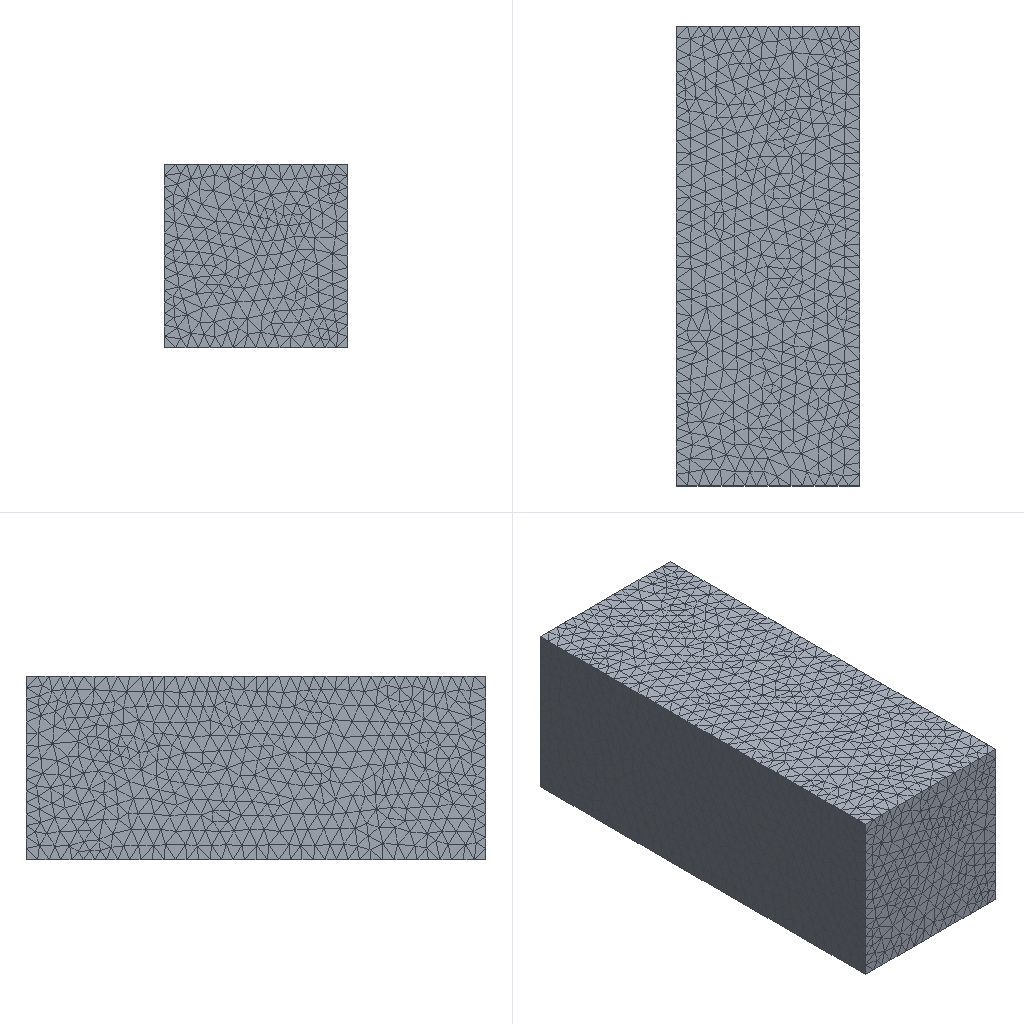Simulation study | ansys workbench
Set-up summary:
category,name,step,type,value,unit,region
solver,ansys_workbench
units,mm-N-s-tonne (MPa),,stated,"/units,MPA"
analysis,LS1,,static
load_step,LS1,LS1,static,nsubst=1; time=1
mesh,nodes,,,44583
mesh,elements,,,30476
element_type,SOLID187,,,22294
element_type,TARGE170,,,3416
element_type,CONTA174,,,3416
element_type,SOLID186,,,948
element_type,SURF154,,,402
material,"? , ABS ( ? )",,E,1628,tonne s^-2 mm^-1
material,"? , ABS ( ? )",,nu,0.4089
material,"? , ABS ( ? )",,density,1.03e-09,tonne mm^-3
material,"? , ABS ( ? )",,conductivity,0.1997,tonne mm s^-3 C^-1
material,"? , ABS ( ? )",,specific_heat,1.4e+09,mm^2 s^-2 C^-1
material,"? , ABS ( ? )",,cte,0.000184,C^-1
material,"? , EN GJL 100",,E,89440,tonne s^-2 mm^-1
material,"? , EN GJL 100",,nu,0.26
material,"? , EN GJL 100",,density,6.999e-09,tonne mm^-3
material,"? , EN GJL 100",,conductivity,60,tonne mm s^-3 C^-1
material,"? , EN GJL 100",,specific_heat,4.996e+08,mm^2 s^-2 C^-1
material,"? , EN GJL 100",,cte,1.196e-05,C^-1
load,Define Force Using Surface Effect Elements,LS1,surface-effect pres face 2,-0.0003125,,SURF154 #15
bc,Fixed Supports,model,fixed,[dofs=ALL],,_FIXEDSU
bc,"Elements for Body 1 ""________|NONE""",model,fixed,[dofs=ALL n=3],,node list
bc,"Elements for Body 2 ""____|____-____1""",model,fixed,[dofs=ALL n=3],,node list
contact,Frictional - ____|____-____1 ? ________|NONE,,standard (frictionless/frictional),friction=0.2; element=CONTA174
contact,Frictional - ____|____-____1 ? ________|NONE,,standard (frictionless/frictional),friction=0.2; element=CONTA174
contact,Frictional - ____|____-____1 ? ________|NONE,,standard (frictionless/frictional),friction=0.2; element=CONTA174
contact,Frictional - ____|____-____1 ? ________|NONE,,standard (frictionless/frictional),friction=0.2; element=CONTA174
contact,Frictional - ____|____-____1 ? ________|NONE,,standard (frictionless/frictional),friction=0.2; element=CONTA174
contact,Frictional - ____|____-____1 ? ________|NONE,,standard (frictionless/frictional),friction=0.2; element=CONTA174
named_set,_FIXEDSU,,node,877
Ansys APDL input file, long lists of numbers shortened:
/batch
/config,noeldb,1     ! force off writing results to database
*get,_wallstrt,active,,time,wall
! ANSYS input file written by Workbench version 2021 R1
! File used for geometry attach:
/title,wbnew--____ (A5)
! ****** Begin Custom Load Command Snippet ******
/COM, ACT Extensions:
/COM,     LSDYNA, 2021.1
/COM,
! ****** End   Custom Load Command Snippet ******
*DIM,_wb_ProjectScratch_dir,string,248
_wb_ProjectScratch_dir(1) = ''
*DIM,_wb_SolverFiles_dir,string,248
_wb_SolverFiles_dir(1) = ''
*DIM,_wb_userfiles_dir,string,248
_wb_userfiles_dir(1) = ''
/com,--- Data in consistent NMM units. See Solving Units in the help system for more information.
/units,MPA
/nopr
/wb,file,start              !  signify a WB generated input file
/prep7
! Turn off shape checking because checks already performed inside WB mesher.
! See help system for more information.
SHPP,OFF,,NOWARN
/nolist
etcon,set             ! allow ANSYS to choose best KEYOP's for 180x elements, resets any applicable keyopt to MAPDL defaults
/com,*********** Nodes for the whole assembly ***********
nblock,3,,49041
(1i9,3e20.9e3)
        1     2.921746114E+01     1.392875542E+01     3.000000000E+01
! (44582 more lines like these left out)
-1
/wb,elem,start            !  set before creation of elements
/com,*********** Elements for Body 1 "________|NONE" ***********
et,1,187
eblock,19,solid,,22294
(19i9)
        1        1        1        1        0        0        0        0       10        0      949     8227     8267    12768    12354    21057    21282    21066    21062
! (44587 more lines like these left out)
-1
/com,*********** Elements for Body 2 "____|____-____1" ***********
et,2,186
keyo,2,2,1          ! set full integration on SOLID186
eblock,19,solid,,948
(19i9)
        2        2        2        2        0        0        0        0       20        0        1     1022     1133     1122     1110     1108     1144     1121     1109
! (1895 more lines like these left out)
-1
/wb,elem,end               !  done creating elements
/com,*********** Send User Defined Coordinate System(s) ***********
csys,0
toffst,273.15,  ! Temperature offset from absolute zero
/com,*********** Set Reference Temperature ***********
tref,22.
/wb,mat,start              !  starting to send materials
/com,*********** Send Materials ***********
Temperature = 'TEMP' ! Temperature
MP,DENS,1,1.03e-09,	! tonne mm^-3
MP,EX,1,1628,	! tonne s^-2 mm^-1
MP,NUXY,1,0.4089,
MP,ALPX,1,0.000184,	! C^-1
MP,KXX,1,0.1997,	! tonne mm s^-3 C^-1
MP,C,1,1400000000,	! mm^2 s^-2 C^-1
Temperature = 'TEMP' ! Temperature
MP,DENS,2,6.999e-09,	! tonne mm^-3
MP,EX,2,89440,	! tonne s^-2 mm^-1
MP,NUXY,2,0.26,
MP,ALPX,2,1.196e-05,	! C^-1
MP,KXX,2,60,	! tonne mm s^-3 C^-1
MP,C,2,499600000,	! mm^2 s^-2 C^-1
/wb,mat,end                !  done sending materials
!************************* Model Summary ********************
!________|NONE,	塑性，ABS（高冲击）,	matid,	1
!____|____-____1,	铸铁，EN GJL 100,	matid,	2
!************************* End Model Summary ********************
! get the diagonal of the bounding box. Needed later for other things
*get,_xmin,node,,mnloc,x
*get,_ymin,node,,mnloc,y
*get,_zmin,node,,mnloc,z
*get,_xmax,node,,mxloc,x
*get,_ymax,node,,mxloc,y
*get,_zmax,node,,mxloc,z
_ASMDIAG=(_xmax-_xmin)*(_xmax-_xmin)+(_ymax-_ymin)*(_ymax-_ymin)+(_zmax-_zmin)*(_zmax-_zmin)
_ASMDIAG=SQRT(_ASMDIAG)
/wb,contact,start          !  starting to send contact
/com,*********** Create Contact "摩擦的 - ____|____-____1 至 ________|NONE" ***********
/com,            Real Constant Set For Above Contact Is 4 & 3
*set,tid,4
*set,cid,3
r,tid
r,cid
et,tid,170
et,cid,174
eblock,10,,,12
(15i9)
    33019        4        4        4        0     2080      184      160       77     2548     2478     2310     2311
! (11 more lines like these left out)
-1
eblock,10,,,12
(15i9)
    33031        3        3        3        0     2080      184      160       77     2548     2478     2310     2311
! (11 more lines like these left out)
-1
eblock,10,,,226
(15i9)
    33043        3        4        3        0     8203     8226     8229     8229    20864    21048     8229    20865
! (225 more lines like these left out)
-1
eblock,10,,,226
(15i9)
    33269        4        3        4        0     8203     8226     8229     8229    20864    21048     8229    20865
! (225 more lines like these left out)
-1
keyo,cid,8,2               ! auto create asymmetric contact (from Program Controlled setting)
keyo,cid,10,0              ! adjust contact stiffness each NR iteration (from Program Controlled setting)
keyo,cid,12,0              ! standard contact
mp,mu,cid,0.2       ! unitless
keyo,cid,18,1              ! small sliding turned on by application
keyo,cid,2,0               ! augmented Lagrange (from Program Controlled setting)
keyo,cid,4,0               ! on Gauss point (from Program Controlled setting)
keyo,cid,9,0               ! use real geometry with stepped effects
keyo,cid,7,0               ! No Prediction
rmod,tid,3,1.       ! FKN
rmod,tid,5,0.       ! ICONT
rmod,tid,6,0.       ! PINB
rmod,tid,10,0.      ! CNOF
rmod,tid,12,0.      ! FKT
rmod,tid,36,35      ! WB DSID
rmod,cid,3,1.       ! FKN
rmod,cid,5,0.       ! ICONT
rmod,cid,6,0.       ! PINB
rmod,cid,10,0.      ! CNOF
rmod,cid,12,0.      ! FKT
rmod,cid,36,35      ! WB DSID
/com,*********** Create Contact "摩擦的 - ____|____-____1 至 ________|NONE" ***********
/com,            Real Constant Set For Above Contact Is 6 & 5
*set,tid,6
*set,cid,5
r,tid
r,cid
et,tid,170
et,cid,174
eblock,10,,,24
(15i9)
    33495        6        6        6        0      159      161      196      158     2477     2481     2475     2474
! (23 more lines like these left out)
-1
eblock,10,,,24
(15i9)
    33519        5        5        5        0      159      161      196      158     2477     2481     2475     2474
! (23 more lines like these left out)
-1
eblock,10,,,688
(15i9)
    33543        5        6        5        0     8298     8346     8508     8508    21484    21933     8508    21488
! (687 more lines like these left out)
-1
eblock,10,,,688
(15i9)
    34231        6        5        6        0     8298     8346     8508     8508    21484    21933     8508    21488
! (687 more lines like these left out)
-1
keyo,cid,8,2               ! auto create asymmetric contact (from Program Controlled setting)
keyo,cid,10,0              ! adjust contact stiffness each NR iteration (from Program Controlled setting)
keyo,cid,12,0              ! standard contact
mp,mu,cid,0.2       ! unitless
keyo,cid,18,1              ! small sliding turned on by application
keyo,cid,2,0               ! augmented Lagrange (from Program Controlled setting)
keyo,cid,4,0               ! on Gauss point (from Program Controlled setting)
keyo,cid,9,0               ! use real geometry with stepped effects
keyo,cid,7,0               ! No Prediction
rmod,tid,3,1.       ! FKN
rmod,tid,5,0.       ! ICONT
rmod,tid,6,0.       ! PINB
rmod,tid,10,0.      ! CNOF
rmod,tid,12,0.      ! FKT
rmod,tid,36,38      ! WB DSID
rmod,cid,3,1.       ! FKN
rmod,cid,5,0.       ! ICONT
rmod,cid,6,0.       ! PINB
rmod,cid,10,0.      ! CNOF
rmod,cid,12,0.      ! FKT
rmod,cid,36,38      ! WB DSID
/com,*********** Create Contact "摩擦的 - ____|____-____1 至 ________|NONE" ***********
/com,            Real Constant Set For Above Contact Is 8 & 7
*set,tid,8
*set,cid,7
r,tid
r,cid
et,tid,170
et,cid,174
eblock,10,,,12
(15i9)
    34919        8        8        8        0     1122     1110     1109     1121     5247     5244     5245     5267
! (11 more lines like these left out)
-1
eblock,10,,,12
(15i9)
    34931        7        7        7        0     1122     1110     1109     1121     5247     5244     5245     5267
! (11 more lines like these left out)
-1
eblock,10,,,228
(15i9)
    34943        7        8        7        0     8592     8616     8632     8632    23373    23567     8632    23374
! (227 more lines like these left out)
-1
eblock,10,,,228
(15i9)
    35171        8        7        8        0     8592     8616     8632     8632    23373    23567     8632    23374
! (227 more lines like these left out)
-1
keyo,cid,8,2               ! auto create asymmetric contact (from Program Controlled setting)
keyo,cid,10,0              ! adjust contact stiffness each NR iteration (from Program Controlled setting)
keyo,cid,12,0              ! standard contact
mp,mu,cid,0.2       ! unitless
keyo,cid,18,1              ! small sliding turned on by application
keyo,cid,2,0               ! augmented Lagrange (from Program Controlled setting)
keyo,cid,4,0               ! on Gauss point (from Program Controlled setting)
keyo,cid,9,0               ! use real geometry with stepped effects
keyo,cid,7,0               ! No Prediction
rmod,tid,3,1.       ! FKN
rmod,tid,5,0.       ! ICONT
rmod,tid,6,0.       ! PINB
rmod,tid,10,0.      ! CNOF
rmod,tid,12,0.      ! FKT
rmod,tid,36,41      ! WB DSID
rmod,cid,3,1.       ! FKN
rmod,cid,5,0.       ! ICONT
rmod,cid,6,0.       ! PINB
rmod,cid,10,0.      ! CNOF
rmod,cid,12,0.      ! FKT
rmod,cid,36,41      ! WB DSID
/com,*********** Create Contact "摩擦的 - ____|____-____1 至 ________|NONE" ***********
/com,            Real Constant Set For Above Contact Is 10 & 9
*set,tid,10
*set,cid,9
r,tid
r,cid
et,tid,170
et,cid,174
eblock,10,,,24
(15i9)
    35399       10       10       10        0     1146     1133     1144     1145     5292     5291     5312     5313
! (23 more lines like these left out)
-1
eblock,10,,,24
(15i9)
    35423        9        9        9        0     1146     1133     1144     1145     5292     5291     5312     5313
! (23 more lines like these left out)
-1
eblock,10,,,700
(15i9)
    35447        9       10        9        0     8675     8816     8728     8728    23885    24395     8728    23883
! (699 more lines like these left out)
-1
eblock,10,,,700
(15i9)
    36147       10        9       10        0     8675     8816     8728     8728    23885    24395     8728    23883
! (699 more lines like these left out)
-1
keyo,cid,8,2               ! auto create asymmetric contact (from Program Controlled setting)
keyo,cid,10,0              ! adjust contact stiffness each NR iteration (from Program Controlled setting)
keyo,cid,12,0              ! standard contact
mp,mu,cid,0.2       ! unitless
keyo,cid,18,1              ! small sliding turned on by application
keyo,cid,2,0               ! augmented Lagrange (from Program Controlled setting)
keyo,cid,4,0               ! on Gauss point (from Program Controlled setting)
keyo,cid,9,0               ! use real geometry with stepped effects
keyo,cid,7,0               ! No Prediction
rmod,tid,3,1.       ! FKN
rmod,tid,5,0.       ! ICONT
rmod,tid,6,0.       ! PINB
rmod,tid,10,0.      ! CNOF
rmod,tid,12,0.      ! FKT
rmod,tid,36,44      ! WB DSID
rmod,cid,3,1.       ! FKN
rmod,cid,5,0.       ! ICONT
rmod,cid,6,0.       ! PINB
rmod,cid,10,0.      ! CNOF
rmod,cid,12,0.      ! FKT
rmod,cid,36,44      ! WB DSID
/com,*********** Create Contact "摩擦的 - ____|____-____1 至 ________|NONE" ***********
/com,            Real Constant Set For Above Contact Is 12 & 11
*set,tid,12
*set,cid,11
r,tid
r,cid
et,tid,170
et,cid,174
eblock,10,,,79
(15i9)
    36847       12       12       12        0     1108     1144     1121     1109     5243     5268     5245     5242
! (78 more lines like these left out)
-1
eblock,10,,,79
(15i9)
    36926       11       11       11        0     1108     1144     1121     1109     5243     5268     5245     5242
! (78 more lines like these left out)
-1
eblock,10,,,678
(15i9)
    37005       11       12       11        0     7649     7835     7727     7727    17355    18026     7727    17352
! (677 more lines like these left out)
-1
eblock,10,,,678
(15i9)
    37683       12       11       12        0     7649     7835     7727     7727    17355    18026     7727    17352
! (677 more lines like these left out)
-1
keyo,cid,8,2               ! auto create asymmetric contact (from Program Controlled setting)
keyo,cid,10,0              ! adjust contact stiffness each NR iteration (from Program Controlled setting)
keyo,cid,12,0              ! standard contact
mp,mu,cid,0.2       ! unitless
keyo,cid,18,1              ! small sliding turned on by application
keyo,cid,2,0               ! augmented Lagrange (from Program Controlled setting)
keyo,cid,4,0               ! on Gauss point (from Program Controlled setting)
keyo,cid,9,0               ! use real geometry with stepped effects
keyo,cid,7,0               ! No Prediction
rmod,tid,3,1.       ! FKN
rmod,tid,5,0.       ! ICONT
rmod,tid,6,0.       ! PINB
rmod,tid,10,0.      ! CNOF
rmod,tid,12,0.      ! FKT
rmod,tid,36,84      ! WB DSID
rmod,cid,3,1.       ! FKN
rmod,cid,5,0.       ! ICONT
rmod,cid,6,0.       ! PINB
rmod,cid,10,0.      ! CNOF
rmod,cid,12,0.      ! FKT
rmod,cid,36,84      ! WB DSID
/com,*********** Create Contact "摩擦的 - ____|____-____1 至 ________|NONE" ***********
/com,            Real Constant Set For Above Contact Is 14 & 13
*set,tid,14
*set,cid,13
r,tid
r,cid
et,tid,170
et,cid,174
eblock,10,,,79
(15i9)
    38361       14       14       14        0       80       78       82       81     2313     2314     2320     2318
! (78 more lines like these left out)
-1
eblock,10,,,79
(15i9)
    38440       13       13       13        0       80       78       82       81     2313     2314     2320     2318
! (78 more lines like these left out)
-1
eblock,10,,,666
(15i9)
    38519       13       14       13        0     7969     8163     8153     8153    19502    20609     8153    19501
! (665 more lines like these left out)
-1
eblock,10,,,666
(15i9)
    39185       14       13       14        0     7969     8163     8153     8153    19502    20609     8153    19501
! (665 more lines like these left out)
-1
keyo,cid,8,2               ! auto create asymmetric contact (from Program Controlled setting)
keyo,cid,10,0              ! adjust contact stiffness each NR iteration (from Program Controlled setting)
keyo,cid,12,0              ! standard contact
mp,mu,cid,0.2       ! unitless
keyo,cid,18,1              ! small sliding turned on by application
keyo,cid,2,0               ! augmented Lagrange (from Program Controlled setting)
keyo,cid,4,0               ! on Gauss point (from Program Controlled setting)
keyo,cid,9,0               ! use real geometry with stepped effects
keyo,cid,7,0               ! No Prediction
rmod,tid,3,1.       ! FKN
rmod,tid,5,0.       ! ICONT
rmod,tid,6,0.       ! PINB
rmod,tid,10,0.      ! CNOF
rmod,tid,12,0.      ! FKT
rmod,tid,36,86      ! WB DSID
rmod,cid,3,1.       ! FKN
rmod,cid,5,0.       ! ICONT
rmod,cid,6,0.       ! PINB
rmod,cid,10,0.      ! CNOF
rmod,cid,12,0.      ! FKT
rmod,cid,36,86      ! WB DSID
nsel,all
esel,all
/wb,contact,end            !  done creating contacts
/golist
/wb,load,start             !  starting to send loads
/com,*********** Fixed Supports ***********
CMBLOCK,_FIXEDSU,NODE,      877
(8i10)
      7095      7096      7097      7098      7099      7100      7101      7102
! (109 more lines like these left out)
cmsel,s,_FIXEDSU
d,all,all
nsel,all
/com,*********** Define Force Using Surface Effect Elements ***********
local,12,0,0.,0.,0.,0.,0.,0.
csys,0
et,15,154
eblock,10,,,402
(15i9)
    39851       15       15       15       12     9157     9218     9315     9315    27049    27573     9315    27052
! (401 more lines like these left out)
-1
esel,s,type,,15
keyop,15,2,1                ! Apply load in local coordinate system
keyop,15,7,1                ! Use original area so load is constant in large deformation
esel,all
et,16,14             ! spring element type
/com,*********** Construct Weak Springs, Prototype 1 ***********
*set,_delta,11.489
type,16
mat,17
real,17
r,17,4.96398843537226e-006
nsel,all
*get,_nspr,ndmx
_nspr=_nspr+1
esel,s,type,,1
nsle,s,active
*get,_minx,node,0,mnloc,x
*get,_miny,node,0,mnloc,y
*get,_minz,node,0,mnloc,z
*get,_maxx,node,0,mxloc,x
*get,_maxy,node,0,mxloc,y
*get,_maxz,node,0,mxloc,z
*dim,_ntets,arra,8
_ntets(1) = NODE(_minx,_miny,_minz)
_ntets(2) = NODE(_minx,_miny,_maxz)
_ntets(3) = NODE(_minx,_maxy,_minz)
_ntets(4) = NODE(_minx,_maxy,_maxz)
_ntets(5) = NODE(_maxx,_miny,_minz)
_ntets(6) = NODE(_maxx,_miny,_maxz)
_ntets(7) = NODE(_maxx,_maxy,_minz)
_ntets(8) = NODE(_maxx,_maxy,_maxz)
*do,_i,1,8
  n,_nspr,nx(_ntets(_i))+_delta,ny(_ntets(_i)),nz(_ntets(_i))
  e,_ntets(_i),_nspr
  d,_nspr,all
  _nspr=_nspr+1
  n,_nspr,nx(_ntets(_i)),ny(_ntets(_i))+_delta,nz(_ntets(_i))
  e,_ntets(_i),_nspr
  d,_nspr,all
  _nspr=_nspr+1
  n,_nspr,nx(_ntets(_i)),ny(_ntets(_i)),nz(_ntets(_i))+_delta
  e,_ntets(_i),_nspr
  d,_nspr,all
  _nspr=_nspr+1
*enddo
*set,_ntets
nsel,all
esel,all
/com,*********** Construct Weak Springs, Prototype 2 ***********
*set,_delta,9.95
type,16
mat,18
real,18
r,18,2.04515375212186e-004
nsel,all
*get,_nspr,ndmx
_nspr=_nspr+1
esel,s,type,,2
nsle,s,active
*get,_minx,node,0,mnloc,x
*get,_miny,node,0,mnloc,y
*get,_minz,node,0,mnloc,z
*get,_maxx,node,0,mxloc,x
*get,_maxy,node,0,mxloc,y
*get,_maxz,node,0,mxloc,z
*dim,_ntets,arra,8
_ntets(1) = NODE(_minx,_miny,_minz)
_ntets(2) = NODE(_minx,_miny,_maxz)
_ntets(3) = NODE(_minx,_maxy,_minz)
_ntets(4) = NODE(_minx,_maxy,_maxz)
_ntets(5) = NODE(_maxx,_miny,_minz)
_ntets(6) = NODE(_maxx,_miny,_maxz)
_ntets(7) = NODE(_maxx,_maxy,_minz)
_ntets(8) = NODE(_maxx,_maxy,_maxz)
*do,_i,1,8
  n,_nspr,nx(_ntets(_i))+_delta,ny(_ntets(_i)),nz(_ntets(_i))
  e,_ntets(_i),_nspr
  d,_nspr,all
  _nspr=_nspr+1
  n,_nspr,nx(_ntets(_i)),ny(_ntets(_i))+_delta,nz(_ntets(_i))
  e,_ntets(_i),_nspr
  d,_nspr,all
  _nspr=_nspr+1
  n,_nspr,nx(_ntets(_i)),ny(_ntets(_i)),nz(_ntets(_i))+_delta
  e,_ntets(_i),_nspr
  d,_nspr,all
  _nspr=_nspr+1
*enddo
*set,_ntets
nsel,all
esel,all
/gst,on,on
fini
*get,_numnode,node,0,count
*get,_numelem,elem,0,count
*get, _MAXELEMNUM, elem, 0, NUM, MAX
*get, _MAXNODENUM, node, 0, NUM, MAX
*get, _MAXELEMTYPE, etyp, 0, NUM, MAX
*get, _MAXREALCONST, real, 0, NUM, MAX
/go
/wb,load,end               !  done creating loads
/com,--- Number of total nodes = %_numnode%
/com,--- Number of contact elements = 7234
/com,--- Number of spring elements = 48
/com,--- Number of bearing elements = 0
/com,--- Number of solid elements = 23242
/com,--- Number of condensed parts = 0
/com,--- Number of total elements = %_numelem%
*get,_wallbsol,active,,time,wall
/com,****************************************************************************
/com,*************************    SOLUTION       ********************************
/com,****************************************************************************
/solu
antype,0                   ! static analysis
_thickRatio=0.5     ! Ratio of thick parts in the model
eqsl,sparse,,,,,1
cntr,print,1               ! print out contact info and also make no initial contact an error
dmpoption,emat,no             ! Don't combine emat file for DANSYS
dmpoption,esav,no             ! Don't combine esav file for DANSYS
nldiag,cont,iter           ! print out contact info each equilibrium iteration
rescontrol,define,last,last,,dele	   ! Program Controlled
/com,****************************************************
/com,******************* SOLVE FOR LS 1 OF 1 ****************
esel,s,type,,15
nsle
sfe,all,1,pres,1,0.
sfe,all,2,pres,1,-3.12499999999906e-004
sfe,all,3,pres,1,0.
nsel,all
esel,all
/nopr
/gopr
/nolist
autots,on                  ! Workbench Program Controlled automatic time stepping
nsub,1,10,1                ! due to presence of general nonlinear
time,1.
outres,erase
outres,all,none
outres,nsol,all,
outres,rsol,all
outres,eangl,all
outres,etmp,all
outres,veng,all
outres,strs,all,
outres,epel,all,
outres,eppl,all,
outres,cont,all,
! *********** WB SOLVE COMMAND ***********
! check interactive state
*get,ANSINTER_,active,,int
*if,ANSINTER_,ne,0,then
/eof
*endif
solve
/com *************** Write FE CONNECTORS *********
CEWRITE,file,ce,,INTE
/com,****************************************************
/com,*************** FINISHED SOLVE FOR LS 1 *************
*get,_wallasol,active,,time,wall
/nopr
*get,_numnode,node,0,count
*get,_numelem,elem,0,count
*get, _MAXELEMNUM, elem, 0, NUM, MAX
*get, _MAXNODENUM, node, 0, NUM, MAX,,,INTERNAL
*get, _MAXELEMTYPE, etyp, 0, NUM, MAX
*get, _MAXREALCONST, real, 0, NUM, MAX
/gopr
/post1
xmlo,ENCODING,ISO-8859-1
xmlo,parm
/xml,parm,xml
fini
/gopr
*get,_walldone,active,,time,wall
_preptime=(_wallbsol-_wallstrt)*3600
_solvtime=(_wallasol-_wallbsol)*3600
_posttime=(_walldone-_wallasol)*3600
_totaltim=(_walldone-_wallstrt)*3600
*get,_dlbratio,active,0,solu,dlbr
*get,_combtime,active,0,solu,comb
/com,--- Total number of nodes = %_numnode%
/com,--- Total number of elements = %_numelem%
/com,--- Element load balance ratio = %_dlbratio%
/com,--- Time to combine distributed files = %_combtime%
/wb,file,end               ! done with WB generated input
Results summary:
result,analyses[0].index,,,1
result,analyses[0].system,,,SYS
result,analyses[0].deck,,,deck.dat
result,analyses[0].solve_status,,,completed
result,analyses[0].analysis_type,,,static
result,analyses[0].physics,,,mechanical
result,analyses[0].unit_system,,,"NMM: mm, ton, N, s, mV, mA, degC"
result,analyses[0].n_sets,,,1
result,analyses[0].load_steps[0].set,set=1,,1
result,analyses[0].load_steps[0].time_or_freq,set=1,,1
result,analyses[0].load_steps[0].max_displacement_magnitude,set=1,,0.0001849
result,analyses[0].load_steps[0].max_von_mises_nodal,set=1,,0.00281
result,analyses[0].load_steps[0].reaction_force_sum_xyz[1],set=1,,-3.5504e-13
result,analyses[0].load_steps[0].reaction_force_sum_xyz[2],set=1,,2
result,analyses[0].load_steps[0].reaction_force_sum_xyz[3],set=1,,-1.5089e-12
result,geometry_export[0][0],,,.step
result,geometry_export[0][1],,,ok
result,geometry_export[0][2],,,2